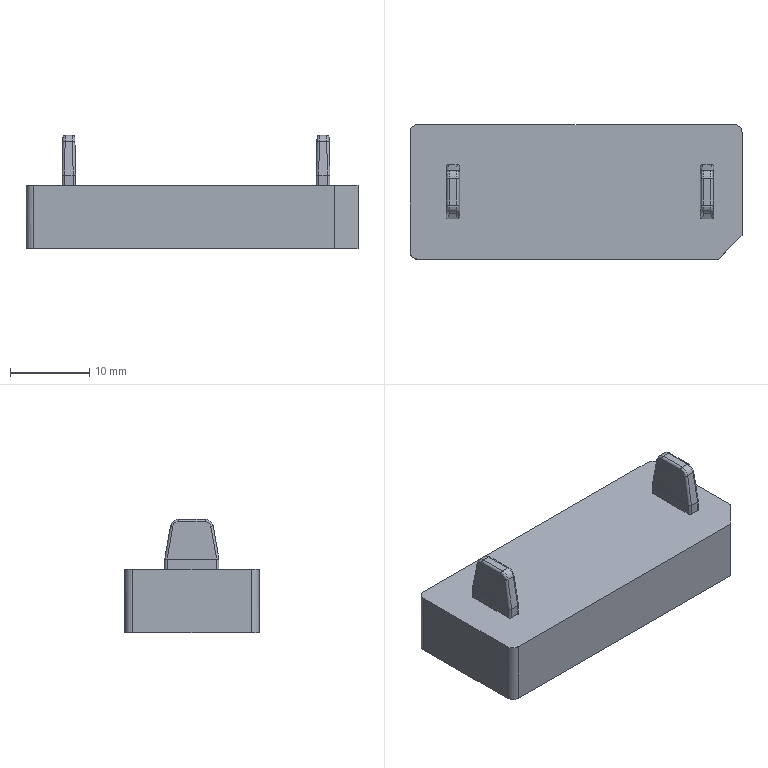NC program | PowerMill | posted by the shop | part box 42 x 17 x 14.346 mm
Lines 1 to 1527 of 86217:
%
G40 G49 G17 G80
( TOOL ID   D10C_1_1 )
( TOOL DIA. 10. TIP RAD 0 LENGTH 69.8 )
( Z = -.074 )
T1 M6
T3
G91 G28 Z0
G0 G90 G54
M08
S8000 M3
G0 X0 Y0 M8
G43 Z10.2 H1
X28.78 Y11.28
Z1.126
G1 Z-.074 F6000
X23.78 F10000
X-23.78
Y5.64
X23.78
Y0
X-23.78
Y-5.64
X23.78
Y-11.28
X-23.78
X-28.78
G0 Z10.2
X.5 Y0
Z9.876
X-29.479 Y-7.144
Z.686
G1 Z-.514 F6000
X-28.951 F10000
G3 X-24.204 Y-2.396 I0 J4.747
G1 Y10.28
G2 X-23.204 Y11.28 I1. J0
G1 X24.204
G2 X25.204 Y10.28 I0 J-1.
G1 Y2.39
X22.604 Y2.224
X22.622 Y1.934
X22.621 Y-1.934
X22.568 Y-2.707
X22.424 Y-3.48
X22.163 Y-4.254
X21.775 Y-5.027
X21.383 Y-5.594
X21.209 Y-5.801
X20.609 Y-6.388
X20.38 Y-6.574
X19.836 Y-6.946
X18.994 Y-7.348
X18.289 Y-7.566
X17.515 Y-7.693
X15.969 Y-7.711
X15.195 Y-7.633
X14.422 Y-7.439
X13.648 Y-7.122
X12.875 Y-6.648
X12.101 Y-5.965
X11.95 Y-5.801
X11.385 Y-5.027
X10.997 Y-4.254
X10.735 Y-3.48
X10.592 Y-2.707
X10.555 Y-2.293
X10.542 Y1.934
X10.587 Y2.707
X10.725 Y3.48
X10.981 Y4.254
X11.328 Y4.969
X11.917 Y5.801
X12.101 Y6.004
X12.875 Y6.686
X13.648 Y7.161
X14.422 Y7.476
X15.195 Y7.673
X15.969 Y7.752
X17.515 Y7.731
X18.289 Y7.605
X19.062 Y7.361
X19.836 Y6.984
X20.609 Y6.427
X21.243 Y5.801
X21.383 Y5.633
X21.799 Y5.027
X22.156 Y4.31
X22.435 Y3.48
X22.573 Y2.707
X22.604 Y2.224
X25.204 Y2.39
Y-10.28
G2 X24.204 Y-11.28 I-1. J0
G1 X-23.204
G2 X-24.204 Y-10.28 I0 J1.
G1 Y-2.396
X-21.599 Y-2.224
X-21.618 Y-1.934
X-21.619 Y1.934
X-21.573 Y2.707
X-21.435 Y3.48
X-21.179 Y4.254
X-20.798 Y5.027
X-20.383 Y5.633
X-20.243 Y5.801
X-19.609 Y6.427
X-19.431 Y6.574
X-18.836 Y6.984
X-18.062 Y7.361
X-17.289 Y7.605
X-16.515 Y7.731
X-14.969 Y7.752
X-14.195 Y7.673
X-13.422 Y7.476
X-13.065 Y7.348
X-12.648 Y7.161
X-11.875 Y6.686
X-11.101 Y6.004
X-10.917 Y5.801
X-10.362 Y5.027
X-9.981 Y4.254
X-9.725 Y3.48
X-9.588 Y2.707
X-9.555 Y2.332
X-9.548 Y-.007
X-3.901 Y-.005
X-3.902 Y3.516
G2 X-1.904 Y5.516 I2. J.001
G1 X2.893 Y5.521
G2 X4.895 Y3.526 I.002 J-2.
G1 X4.91 Y-3.513
G2 X2.913 Y-5.518 I-2. J-.004
G1 X-1.896 Y-5.525
G2 X-3.899 Y-3.526 I-.003 J2.
G1 X-3.901 Y-.005
X-9.548 Y-.007
X-9.542 Y-1.934
X-9.592 Y-2.707
X-9.735 Y-3.48
X-9.997 Y-4.254
X-10.328 Y-4.93
X-10.951 Y-5.801
X-11.101 Y-5.965
X-11.78 Y-6.574
X-12.648 Y-7.122
X-13.166 Y-7.348
X-13.422 Y-7.439
X-14.195 Y-7.633
X-14.969 Y-7.711
X-16.515 Y-7.693
X-17.289 Y-7.566
X-17.991 Y-7.348
X-18.836 Y-6.946
X-19.381 Y-6.574
X-19.609 Y-6.388
X-20.209 Y-5.801
X-20.383 Y-5.594
X-20.775 Y-5.027
X-21.156 Y-4.271
X-21.425 Y-3.48
X-21.567 Y-2.707
X-21.599 Y-2.224
X-24.204 Y-2.396
G0 Z3.296
G1 X-29.479 Y-7.144
G0 Z.296
G1 Z-.904 F6000
X-28.951 F10000
G3 X-24.204 Y-2.396 I0 J4.747
G1 Y0
X-21.619
Y1.934
X-21.618 Y1.951
Y2.707
X-21.512 Y3.48
X-21.3 Y4.254
X-21.156 Y4.618
X-20.953 Y5.027
X-20.45 Y5.801
X-19.722 Y6.574
X-18.836 Y7.208
X-18.581 Y7.348
X-18.062 Y7.581
X-17.289 Y7.817
X-16.515 Y7.942
X-14.969 Y7.961
X-14.195 Y7.883
X-13.422 Y7.694
X-12.648 Y7.383
X-11.875 Y6.917
X-11.438 Y6.574
X-11.101 Y6.255
X-10.71 Y5.801
X-10.207 Y5.027
X-9.859 Y4.254
X-9.649 Y3.48
X-9.555 Y2.861
X-9.531 Y1.934
X-9.537 Y.059
X-3.793 Y.021
X-3.77 Y3.553
G2 X-1.762 Y5.54 I2. J-.013
G1 X2.819 Y5.522
G2 X4.811 Y3.531 I-.008 J-2.
G1 X4.842 Y-3.501
G2 X2.849 Y-5.51 I-2. J-.009
G1 X-1.81 Y-5.526
G2 X-3.817 Y-3.512 I-.007 J2.
G1 X-3.793 Y.021
X-9.537 Y.059
X-9.543 Y-1.621
X-9.542 Y-1.934
X-9.544 Y-1.967
X-9.547 Y-2.707
X-9.657 Y-3.48
X-9.873 Y-4.254
X-10.229 Y-5.027
X-10.741 Y-5.801
X-11.101 Y-6.215
X-11.484 Y-6.574
X-11.875 Y-6.876
X-12.656 Y-7.348
X-13.422 Y-7.655
X-14.195 Y-7.844
X-14.969 Y-7.921
X-16.515 Y-7.903
X-17.289 Y-7.777
X-18.062 Y-7.542
X-18.503 Y-7.348
X-18.836 Y-7.168
X-19.609 Y-6.63
X-20.383 Y-5.847
X-20.931 Y-5.027
X-21.156 Y-4.578
X-21.287 Y-4.254
X-21.504 Y-3.48
X-21.615 Y-2.707
Y-1.986
X-21.618 Y-1.934
X-21.619 Y0
X-24.204
Y10.28
G2 X-23.204 Y11.28 I1. J0
G1 X24.204
G2 X25.204 Y10.28 I0 J-1.
G1 Y2.706
X22.616 Y2.707
Y2.024
X22.622 Y1.934
X22.621 Y-1.934
X22.615 Y-2.015
Y-2.707
X22.503 Y-3.48
X22.285 Y-4.254
X22.156 Y-4.578
X21.931 Y-5.027
X21.419 Y-5.801
X20.676 Y-6.574
X19.836 Y-7.168
X19.504 Y-7.348
X19.062 Y-7.542
X18.289 Y-7.778
X17.515 Y-7.903
X15.969 Y-7.921
X15.195 Y-7.844
X14.422 Y-7.655
X13.656 Y-7.348
X12.875 Y-6.876
X12.484 Y-6.574
X12.101 Y-6.215
X11.741 Y-5.801
X11.229 Y-5.027
X10.873 Y-4.254
X10.657 Y-3.48
X10.545 Y-2.707
X10.543 Y1.887
X10.542 Y1.934
X10.543 Y1.935
X10.542 Y2.707
X10.648 Y3.48
X10.859 Y4.254
X11.207 Y5.027
X11.71 Y5.801
X12.101 Y6.255
X12.438 Y6.574
X12.875 Y6.917
X13.579 Y7.348
X14.422 Y7.694
X15.195 Y7.883
X15.969 Y7.961
X17.515 Y7.942
X18.289 Y7.817
X19.062 Y7.581
X19.582 Y7.348
X19.836 Y7.208
X20.609 Y6.669
X21.383 Y5.887
X21.954 Y5.027
X22.156 Y4.618
X22.301 Y4.254
X22.511 Y3.48
X22.616 Y2.707
X25.204 Y2.706
Y-10.28
G2 X24.204 Y-11.28 I-1. J0
G1 X-23.204
G2 X-24.204 Y-10.28 I0 J1.
G1 Y-2.396
G0 Z2.907
G1 X-29.479 Y-7.144
G0 Z-.093
G1 Z-1.293 F6000
X-28.951 F10000
G3 X-24.204 Y-2.396 I0 J4.747
G1 Y10.28
G2 X-23.204 Y11.28 I1. J0
G1 X24.204
G2 X25.204 Y10.28 I0 J-1.
G1 Y2.706
X22.629 Y2.707
X22.628 Y-2.707
X22.528 Y-3.48
X22.319 Y-4.254
X22.156 Y-4.679
X21.988 Y-5.027
X21.383 Y-5.937
X20.609 Y-6.718
X19.836 Y-7.259
X19.674 Y-7.348
X19.062 Y-7.624
X18.289 Y-7.856
X17.515 Y-7.982
X15.969 Y-8.
X15.195 Y-7.923
X14.422 Y-7.733
X13.648 Y-7.431
X12.875 Y-6.97
X12.388 Y-6.574
X12.101 Y-6.293
X11.669 Y-5.801
X11.328 Y-5.304
X11.172 Y-5.027
X10.841 Y-4.254
X10.632 Y-3.48
X10.532 Y-2.707
X10.53 Y2.707
X10.624 Y3.48
X10.827 Y4.254
X11.152 Y5.027
X11.328 Y5.343
X11.639 Y5.801
X12.101 Y6.333
X12.346 Y6.574
X12.875 Y7.009
X13.413 Y7.348
X13.648 Y7.47
X14.422 Y7.773
X15.195 Y7.962
X15.969 Y8.039
X17.515 Y8.021
X18.289 Y7.895
X19.062 Y7.663
X19.747 Y7.348
X20.609 Y6.757
X20.814 Y6.574
X21.383 Y5.976
X21.521 Y5.801
X22.008 Y5.027
X22.156 Y4.718
X22.333 Y4.254
X22.535 Y3.48
X22.629 Y2.707
X25.204 Y2.706
Y-10.28
G2 X24.204 Y-11.28 I-1. J0
G1 X-23.204
G2 X-24.204 Y-10.28 I0 J1.
G1 Y-2.708
X-21.628 Y-2.707
X-21.63 Y2.707
X-21.535 Y3.48
X-21.333 Y4.254
X-21.156 Y4.718
X-21.009 Y5.027
X-20.521 Y5.801
X-20.383 Y5.976
X-19.814 Y6.574
X-19.609 Y6.757
X-18.836 Y7.298
X-18.062 Y7.663
X-17.289 Y7.895
X-16.515 Y8.021
X-14.969 Y8.039
X-14.195 Y7.962
X-13.422 Y7.773
X-12.648 Y7.47
X-12.413 Y7.348
X-11.875 Y7.009
X-11.346 Y6.574
X-11.101 Y6.333
X-10.639 Y5.801
X-10.328 Y5.343
X-10.152 Y5.027
X-9.827 Y4.254
X-9.624 Y3.48
X-9.53 Y2.707
X-9.531 Y-.021
X-3.807 Y-.011
X-3.813 Y3.501
G2 X-1.817 Y5.505 I2. J.004
G1 X2.793 Y5.515
G2 X4.797 Y3.523 I.004 J-2.
G1 X4.825 Y-3.496
G2 X2.831 Y-5.504 I-2. J-.008
G1 X-1.794 Y-5.519
G2 X-3.801 Y-3.522 I-.007 J2.
G1 X-3.807 Y-.011
X-9.531 Y-.021
X-9.532 Y-2.707
X-9.632 Y-3.48
X-9.841 Y-4.254
X-10.172 Y-5.027
X-10.328 Y-5.304
X-10.669 Y-5.801
X-11.101 Y-6.293
X-11.388 Y-6.574
X-11.875 Y-6.97
X-12.485 Y-7.348
X-13.422 Y-7.733
X-14.195 Y-7.923
X-14.969 Y-8.
X-16.515 Y-7.982
X-17.289 Y-7.856
X-18.062 Y-7.624
X-18.836 Y-7.259
X-19.609 Y-6.718
X-20.383 Y-5.937
X-20.988 Y-5.027
X-21.156 Y-4.679
X-21.32 Y-4.254
X-21.528 Y-3.48
X-21.628 Y-2.707
X-24.204 Y-2.708
Y-2.396
G0 Z2.517
G1 X-29.479 Y-7.144
G0 Z-.483
G1 Z-1.683 F6000
X-28.951 F10000
G3 X-24.204 Y-2.396 I0 J4.747
G1 Y10.28
G2 X-23.204 Y11.28 I1. J0
G1 X24.204
G2 X25.204 Y10.28 I0 J-1.
G1 Y-.001
X22.638 Y0
Y-2.707
X22.548 Y-3.48
X22.348 Y-4.254
X22.156 Y-4.763
X22.03 Y-5.027
X21.55 Y-5.801
X21.383 Y-6.014
X20.852 Y-6.574
X20.609 Y-6.792
X19.807 Y-7.348
X19.062 Y-7.695
X18.289 Y-7.926
X17.515 Y-8.051
X15.969 Y-8.069
X15.195 Y-7.993
X14.422 Y-7.804
X13.648 Y-7.503
X13.353 Y-7.348
X12.875 Y-7.043
X12.308 Y-6.574
X12.101 Y-6.369
X11.61 Y-5.801
X11.328 Y-5.384
X11.13 Y-5.027
X10.812 Y-4.254
X10.613 Y-3.48
X10.555 Y-3.113
X10.523 Y-2.707
X10.521 Y2.707
X10.606 Y3.48
X10.799 Y4.254
X11.11 Y5.027
X11.328 Y5.423
X11.581 Y5.801
X12.267 Y6.574
X12.875 Y7.083
X13.284 Y7.348
X13.648 Y7.542
X14.422 Y7.843
X15.195 Y8.032
X15.969 Y8.108
X17.515 Y8.09
X18.289 Y7.965
X19.062 Y7.734
X19.836 Y7.371
X20.609 Y6.831
X20.893 Y6.574
X21.383 Y6.053
X21.579 Y5.801
X22.05 Y5.027
X22.361 Y4.254
X22.554 Y3.48
X22.639 Y2.707
X22.638 Y0
X25.204 Y-.001
Y-10.28
G2 X24.204 Y-11.28 I-1. J0
G1 X-23.204
G2 X-24.204 Y-10.28 I0 J1.
G1 Y-2.708
X-21.638 Y-2.707
X-21.639 Y2.707
X-21.555 Y3.48
X-21.361 Y4.254
X-21.051 Y5.027
X-20.579 Y5.801
X-20.383 Y6.053
X-19.893 Y6.574
X-19.609 Y6.831
X-18.876 Y7.348
X-18.062 Y7.734
X-17.289 Y7.965
X-16.515 Y8.09
X-14.969 Y8.108
X-14.195 Y8.032
X-13.422 Y7.843
X-12.648 Y7.542
X-12.285 Y7.348
X-11.875 Y7.083
X-11.267 Y6.574
X-10.581 Y5.801
X-10.328 Y5.423
X-10.11 Y5.027
X-9.799 Y4.254
X-9.605 Y3.48
X-9.521 Y2.707
Y-.019
X-3.779 Y-.01
X-3.785 Y3.505
G2 X-1.785 Y5.508 I2. J.003
G1 X2.785
G2 X4.785 Y3.512 I0 J-2.
G1 X4.798 Y-3.503
G2 X2.804 Y-5.506 I-2. J-.004
G1 X-1.767 Y-5.521
G2 X-3.774 Y-3.525 I-.007 J2.
G1 X-3.779 Y-.01
X-9.521 Y-.019
X-9.522 Y-2.707
X-9.555 Y-3.113
X-9.613 Y-3.48
X-9.812 Y-4.254
X-10.13 Y-5.027
X-10.328 Y-5.384
X-10.61 Y-5.801
X-11.101 Y-6.369
X-11.307 Y-6.574
X-11.875 Y-7.043
X-12.354 Y-7.348
X-12.648 Y-7.503
X-13.422 Y-7.804
X-14.195 Y-7.993
X-14.969 Y-8.069
X-16.515 Y-8.051
X-17.289 Y-7.926
X-18.062 Y-7.695
X-18.836 Y-7.332
X-19.609 Y-6.792
X-19.852 Y-6.574
X-20.383 Y-6.014
X-20.55 Y-5.801
X-21.03 Y-5.027
X-21.156 Y-4.763
X-21.348 Y-4.254
X-21.548 Y-3.48
X-21.638 Y-2.707
X-24.204 Y-2.708
Y-2.396
G0 Z2.127
G1 X-29.479 Y-7.144
G0 Z-.873
G1 Z-2.073 F6000
X-28.951 F10000
G3 X-24.204 Y-2.396 I0 J4.747
G1 Y10.28
G2 X-23.204 Y11.28 I1. J0
G1 X24.204
G2 X25.204 Y10.28 I0 J-1.
G1 Y-.001
X22.648 Y0
X22.646 Y-2.707
X22.567 Y-3.48
X22.376 Y-4.254
X22.072 Y-5.027
X21.607 Y-5.801
X21.383 Y-6.09
X20.929 Y-6.574
X20.609 Y-6.866
X19.932 Y-7.348
X19.062 Y-7.766
X18.289 Y-7.996
X17.505 Y-8.121
X15.969 Y-8.138
X15.195 Y-8.062
X14.422 Y-7.875
X13.648 Y-7.575
X13.228 Y-7.348
X12.875 Y-7.117
X12.23 Y-6.574
X11.553 Y-5.801
X11.328 Y-5.463
X11.088 Y-5.027
X10.784 Y-4.254
X10.594 Y-3.48
X10.557 Y-3.128
X10.555 Y-3.113
X10.552 Y-3.08
X10.513 Y-2.707
Y-.033
X4.734 Y-.012
X4.722 Y-3.538
G2 X2.71 Y-5.531 I-2. J.007
G1 X-1.787 Y-5.505
G2 X-3.776 Y-3.505 I.011 J2.
G1 X-3.773 Y3.502
G2 X-1.782 Y5.501 I2. J-.001
G1 X2.739 Y5.521
G2 X4.747 Y3.513 I.009 J-2.
G1 X4.734 Y-.012
X10.513 Y-.033
X10.512 Y2.707
X10.555 Y3.275
X10.771 Y4.254
X11.069 Y5.027
X11.328 Y5.503
X11.525 Y5.801
X12.101 Y6.484
X12.875 Y7.156
X13.164 Y7.348
X13.648 Y7.614
X14.422 Y7.914
X15.195 Y8.102
X15.969 Y8.177
X17.515 Y8.159
X18.289 Y8.035
X19.062 Y7.805
X19.836 Y7.444
X20.609 Y6.906
X20.968 Y6.574
X21.383 Y6.129
X21.635 Y5.801
X22.091 Y5.027
X22.389 Y4.254
X22.574 Y3.48
X22.649 Y2.707
X22.648 Y0
X25.204 Y-.001
Y-10.28
G2 X24.204 Y-11.28 I-1. J0
G1 X-23.204
G2 X-24.204 Y-10.28 I0 J1.
G1 Y-2.707
X-21.647
X-21.648 Y2.707
X-21.574 Y3.48
X-21.389 Y4.254
X-21.156 Y4.886
X-20.635 Y5.801
X-20.383 Y6.129
X-19.969 Y6.574
X-19.609 Y6.906
X-18.836 Y7.444
X-18.062 Y7.805
X-17.289 Y8.035
X-16.515 Y8.159
X-14.969 Y8.177
X-14.315 Y8.121
X-13.422 Y7.914
X-12.648 Y7.614
X-12.163 Y7.348
X-11.875 Y7.156
X-11.192 Y6.574
X-10.525 Y5.801
X-10.328 Y5.503
X-10.069 Y5.027
X-9.771 Y4.254
X-9.586 Y3.48
X-9.511 Y2.707
X-9.512 Y-2.707
X-9.554 Y-3.099
X-9.555 Y-3.113
X-9.556 Y-3.119
X-9.593 Y-3.48
X-9.783 Y-4.254
X-10.088 Y-5.027
X-10.328 Y-5.463
X-10.553 Y-5.801
X-11.101 Y-6.445
X-11.875 Y-7.117
X-12.228 Y-7.348
X-12.648 Y-7.575
X-13.422 Y-7.875
X-14.195 Y-8.062
X-14.654 Y-8.121
X-14.969 Y-8.138
X-16.505 Y-8.121
X-17.289 Y-7.996
X-18.062 Y-7.766
X-18.836 Y-7.404
X-19.609 Y-6.866
X-19.929 Y-6.574
X-20.383 Y-6.09
X-20.607 Y-5.801
X-21.071 Y-5.027
X-21.377 Y-4.254
X-21.567 Y-3.48
X-21.647 Y-2.707
X-24.204
Y-2.396
G0 Z1.737
G1 X-29.479 Y-7.144
G0 Z-1.263
G1 Z-2.463 F6000
X-28.951 F10000
G3 X-24.204 Y-2.396 I0 J4.747
G1 Y0
X-21.656
Y2.707
X-21.592 Y3.48
X-21.415 Y4.254
X-21.156 Y4.97
X-20.691 Y5.801
X-20.383 Y6.206
X-20.044 Y6.574
X-19.609 Y6.98
X-19.111 Y7.348
X-18.836 Y7.516
X-18.062 Y7.877
X-17.289 Y8.106
X-16.515 Y8.229
X-14.969 Y8.246
X-14.195 Y8.172
X-13.422 Y7.985
X-12.648 Y7.686
X-11.875 Y7.23
X-11.101 Y6.56
X-10.47 Y5.801
X-10.328 Y5.582
X-10.031 Y5.027
X-9.745 Y4.254
X-9.567 Y3.48
X-9.504 Y2.707
Y-2.707
X-9.555 Y-3.355
X-9.756 Y-4.254
X-10.049 Y-5.027
X-10.328 Y-5.543
X-10.497 Y-5.801
X-11.101 Y-6.52
X-11.875 Y-7.19
X-12.109 Y-7.348
X-12.648 Y-7.647
X-13.422 Y-7.946
X-14.132 Y-8.121
X-14.969 Y-8.206
X-16.515 Y-8.189
X-17.289 Y-8.067
X-18.062 Y-7.837
X-18.836 Y-7.477
X-19.051 Y-7.348
X-19.609 Y-6.941
X-20.005 Y-6.574
X-20.383 Y-6.167
X-20.663 Y-5.801
X-21.111 Y-5.027
X-21.405 Y-4.254
X-21.586 Y-3.48
X-21.656 Y-2.707
Y0
X-24.204
Y10.28
G2 X-23.204 Y11.28 I1. J0
G1 X24.204
G2 X25.204 Y10.28 I0 J-1.
G1 Y0
X22.656
X22.655 Y-2.707
X22.586 Y-3.48
X22.405 Y-4.254
X22.156 Y-4.931
X21.663 Y-5.801
X21.383 Y-6.167
X21.005 Y-6.574
X20.609 Y-6.941
X20.051 Y-7.348
X19.836 Y-7.477
X19.062 Y-7.837
X18.289 Y-8.067
X18.028 Y-8.121
X17.515 Y-8.189
X15.969 Y-8.206
X15.195 Y-8.132
X14.422 Y-7.946
X13.648 Y-7.647
X13.109 Y-7.348
X12.875 Y-7.19
X12.155 Y-6.574
X11.497 Y-5.801
X11.328 Y-5.543
X11.049 Y-5.027
X10.755 Y-4.254
X10.575 Y-3.48
X10.504 Y-2.707
Y.089
X4.73 Y.033
X4.764 Y-3.479
G2 X2.764 Y-5.498 I-2. J-.019
G1 X-1.769
G2 X-3.769 Y-3.496 I0 J2.
G1 X-3.762 Y3.496
G2 X-1.776 Y5.494 I2. J-.002
G1 X2.682 Y5.525
G2 X4.696 Y3.545 I.014 J-2.
G1 X4.73 Y.033
X10.504 Y.089
Y2.707
X10.555 Y3.395
X10.745 Y4.254
X11.031 Y5.027
X11.328 Y5.582
X11.47 Y5.801
X12.101 Y6.56
X12.875 Y7.23
X13.648 Y7.686
X14.422 Y7.985
X15.195 Y8.172
X15.969 Y8.246
X17.515 Y8.229
X18.222 Y8.121
X19.062 Y7.877
X19.836 Y7.516
X20.112 Y7.348
X20.609 Y6.98
X21.043 Y6.574
X21.383 Y6.206
X21.69 Y5.801
X22.13 Y5.027
X22.415 Y4.254
X22.592 Y3.48
X22.656 Y2.707
Y0
X25.204
Y-10.28
G2 X24.204 Y-11.28 I-1. J0
G1 X-23.204
G2 X-24.204 Y-10.28 I0 J1.
G1 Y-2.396
G0 Z1.348
G1 X-29.479 Y-7.144
G0 Z-1.652
G1 Z-2.852 F6000
X-28.951 F10000
G3 X-24.204 Y-2.396 I0 J4.747
G1 Y10.28
G2 X-23.204 Y11.28 I1. J0
G1 X24.204
G2 X25.204 Y10.28 I0 J-1.
G1 Y0
X22.663
Y-2.707
X22.603 Y-3.48
X22.43 Y-4.254
X22.156 Y-5.015
X21.717 Y-5.801
X21.383 Y-6.244
X21.079 Y-6.574
X20.609 Y-7.015
X20.163 Y-7.348
X19.836 Y-7.549
X19.062 Y-7.909
X18.354 Y-8.121
X17.515 Y-8.259
X15.969 Y-8.275
X15.195 Y-8.202
X14.422 Y-8.016
X13.648 Y-7.719
X12.996 Y-7.348
X12.101 Y-6.596
X11.443 Y-5.801
X11.01 Y-5.027
X10.73 Y-4.254
X10.556 Y-3.48
X10.497 Y-2.707
Y2.707
X10.555 Y3.51
X10.719 Y4.254
X10.992 Y5.027
X11.417 Y5.801
X12.042 Y6.574
X12.875 Y7.303
X13.648 Y7.758
X14.422 Y8.056
X15.195 Y8.241
X15.969 Y8.314
X17.515 Y8.298
X18.289 Y8.176
X19.062 Y7.948
X19.836 Y7.589
X20.221 Y7.348
X20.609 Y7.054
X21.117 Y6.574
X21.383 Y6.283
X21.743 Y5.801
X22.156 Y5.054
X22.441 Y4.254
X22.609 Y3.48
X22.663 Y2.707
Y0
X25.204
Y-10.28
G2 X24.204 Y-11.28 I-1. J0
G1 X-23.204
G2 X-24.204 Y-10.28 I0 J1.
G1 Y-2.707
X-21.663
Y2.707
X-21.609 Y3.48
X-21.441 Y4.254
X-21.168 Y5.027
X-20.743 Y5.801
X-20.383 Y6.283
X-20.118 Y6.574
X-19.609 Y7.054
X-19.221 Y7.348
X-18.836 Y7.589
X-18.062 Y7.948
X-17.289 Y8.176
X-16.515 Y8.298
X-14.969 Y8.314
X-14.195 Y8.241
X-13.422 Y8.056
X-12.648 Y7.758
X-11.939 Y7.348
X-11.101 Y6.635
X-10.417 Y5.801
X-9.993 Y5.027
X-9.72 Y4.254
X-9.555 Y3.51
X-9.497 Y2.707
Y-.045
X-3.691 Y-.021
X-3.705 Y3.491
G2 X-1.707 Y5.515 I2. J.024
G1 X2.676 Y5.52
G2 X4.678 Y3.541 I.002 J-2.
G1 X4.753 Y-3.47
G2 X2.77 Y-5.491 I-2. J-.021
G1 X-1.659 Y-5.528
G2 X-3.676 Y-3.533 I-.017 J2.
G1 X-3.691 Y-.021
X-9.497 Y-.045
Y-2.707
X-9.555 Y-3.471
X-9.729 Y-4.254
X-10.011 Y-5.027
X-10.443 Y-5.801
X-11.101 Y-6.596
X-11.875 Y-7.264
X-12.648 Y-7.719
X-13.422 Y-8.016
X-13.807 Y-8.121
X-14.195 Y-8.202
X-14.969 Y-8.275
X-16.515 Y-8.259
X-17.289 Y-8.137
X-18.062 Y-7.909
X-18.836 Y-7.549
X-19.164 Y-7.348
X-19.609 Y-7.015
X-20.08 Y-6.574
X-20.383 Y-6.244
X-20.716 Y-5.801
X-21.15 Y-5.027
X-21.43 Y-4.254
X-21.604 Y-3.48
X-21.663 Y-2.707
X-24.204
Y-2.396
G0 Z.958
G1 X-29.479 Y-7.144
G0 Z-2.042
G1 Z-3.242 F6000
X-28.951 F10000
G3 X-24.204 Y-2.396 I0 J4.747
G1 Y10.28
G2 X-23.204 Y11.28 I1. J0
G1 X24.204
G2 X25.204 Y10.28 I0 J-1.
G1 Y0
X22.67
Y-2.707
X22.62 Y-3.48
X22.455 Y-4.254
X22.187 Y-5.027
X21.769 Y-5.801
X21.383 Y-6.321
X21.153 Y-6.574
X20.609 Y-7.089
X20.27 Y-7.348
X19.836 Y-7.622
X19.062 Y-7.98
X18.618 Y-8.121
X18.289 Y-8.207
X17.515 Y-8.328
X15.969 Y-8.344
X15.195 Y-8.272
X14.542 Y-8.121
X13.648 Y-7.79
X12.89 Y-7.348
X12.101 Y-6.672
X11.39 Y-5.801
X10.973 Y-5.027
X10.704 Y-4.254
X10.555 Y-3.584
X10.49 Y-2.707
Y2.707
X10.535 Y3.48
X10.694 Y4.254
X10.956 Y5.027
X11.328 Y5.741
X11.969 Y6.574
X12.834 Y7.348
X13.648 Y7.83
X14.404 Y8.121
X15.195 Y8.311
X15.969 Y8.383
X17.515 Y8.367
X18.289 Y8.246
X19.062 Y8.019
X19.836 Y7.661
X20.326 Y7.348
X20.609 Y7.129
X21.191 Y6.574
X21.383 Y6.36
X21.795 Y5.801
X22.156 Y5.138
X22.466 Y4.254
X22.626 Y3.48
X22.67 Y2.707
Y0
X25.204
Y-10.28
G2 X24.204 Y-11.28 I-1. J0
G1 X-23.204
G2 X-24.204 Y-10.28 I0 J1.
G1 Y-3.163
X-21.651 Y-2.997
X-21.67 Y-2.707
Y2.707
X-21.626 Y3.48
X-21.466 Y4.254
X-21.204 Y5.027
X-20.795 Y5.801
X-20.383 Y6.36
X-20.191 Y6.574
X-19.609 Y7.129
X-19.326 Y7.348
X-18.836 Y7.661
X-18.062 Y8.019
X-17.289 Y8.246
X-16.515 Y8.367
X-14.969 Y8.383
X-14.195 Y8.311
X-13.422 Y8.126
X-12.648 Y7.83
X-11.875 Y7.377
X-10.969 Y6.574
X-10.365 Y5.801
X-9.956 Y5.027
X-9.694 Y4.254
X-9.555 Y3.622
X-9.49 Y2.707
Y-.055
X-3.717 Y-.025
X-3.735 Y3.47
G2 X-1.747 Y5.481 I2. J.01
G1 X2.685 Y5.507
G2 X4.696 Y3.519 I.012 J-2.
G1 X4.739 Y-3.472
G2 X2.751 Y-5.484 I-2. J-.012
G1 X-1.687 Y-5.51
G2 X-3.699 Y-3.521 I-.012 J2.
G1 X-3.717 Y-.025
X-9.49 Y-.055
Y-2.707
X-9.54 Y-3.48
X-9.704 Y-4.254
X-9.972 Y-5.027
X-10.328 Y-5.702
X-11.007 Y-6.574
X-11.875 Y-7.337
X-12.648 Y-7.79
X-13.542 Y-8.121
X-14.195 Y-8.272
X-14.969 Y-8.344
X-16.515 Y-8.328
X-17.289 Y-8.207
X-18.062 Y-7.98
X-18.836 Y-7.622
X-19.27 Y-7.348
X-19.609 Y-7.089
X-20.153 Y-6.574
X-20.383 Y-6.321
X-20.77 Y-5.801
X-21.156 Y-5.099
X-21.456 Y-4.254
X-21.62 Y-3.48
X-21.651 Y-2.997
X-24.204 Y-3.163
Y-2.396
G0 Z.568
G1 X-29.479 Y-7.144
G0 Z-2.432
G1 Z-3.632 F6000
X-28.951 F10000
G3 X-24.204 Y-2.396 I0 J4.747
G1 Y0
X-21.677
Y2.707
X-21.641 Y3.48
X-21.491 Y4.254
X-21.239 Y5.027
X-20.845 Y5.801
X-20.383 Y6.437
X-19.609 Y7.203
X-19.425 Y7.348
X-18.836 Y7.734
X-18.062 Y8.09
X-17.289 Y8.317
X-16.515 Y8.436
X-14.969 Y8.452
X-14.195 Y8.381
X-13.422 Y8.197
X-12.648 Y7.902
X-11.875 Y7.45
X-11.101 Y6.786
X-10.899 Y6.574
X-10.315 Y5.801
X-9.921 Y5.027
X-9.669 Y4.254
X-9.519 Y3.48
X-9.483 Y2.707
Y-2.707
X-9.524 Y-3.48
X-9.679 Y-4.254
X-9.937 Y-5.027
X-10.34 Y-5.801
X-10.935 Y-6.574
X-11.101 Y-6.747
X-11.787 Y-7.348
X-12.648 Y-7.862
X-13.302 Y-8.121
X-14.195 Y-8.342
X-14.969 Y-8.413
X-16.515 Y-8.397
X-17.289 Y-8.277
X-18.062 Y-8.051
X-18.836 Y-7.695
X-19.373 Y-7.348
X-19.609 Y-7.164
X-20.226 Y-6.574
X-20.383 Y-6.397
X-20.82 Y-5.801
X-21.156 Y-5.182
X-21.481 Y-4.254
X-21.636 Y-3.48
X-21.677 Y-2.707
Y0
X-24.204
Y10.28
G2 X-23.204 Y11.28 I1. J0
G1 X24.204
G2 X25.204 Y10.28 I0 J-1.
G1 Y0
X22.677
Y-2.707
X22.637 Y-3.48
X22.48 Y-4.254
X22.223 Y-5.027
X21.82 Y-5.801
X21.383 Y-6.397
X21.225 Y-6.574
X20.609 Y-7.164
X20.374 Y-7.348
X19.836 Y-7.695
X19.062 Y-8.051
X18.858 Y-8.121
X18.289 Y-8.277
X17.515 Y-8.397
X15.969 Y-8.413
X15.195 Y-8.342
X14.422 Y-8.158
X13.648 Y-7.862
X12.875 Y-7.411
X12.101 Y-6.747
X11.935 Y-6.574
X11.34 Y-5.801
X10.937 Y-5.027
X10.679 Y-4.254
X10.524 Y-3.48
X10.483 Y-2.707
Y2.707
X10.52 Y3.48
X10.668 Y4.254
X10.921 Y5.027
X11.315 Y5.801
X11.898 Y6.574
X12.101 Y6.786
X12.875 Y7.45
X13.648 Y7.902
X14.184 Y8.121
X15.195 Y8.381
X15.969 Y8.452
X17.515 Y8.436
X18.289 Y8.317
X18.976 Y8.121
X19.836 Y7.734
X20.426 Y7.348
X20.609 Y7.203
X21.261 Y6.574
X21.845 Y5.801
X22.24 Y5.027
X22.492 Y4.254
X22.64 Y3.48
X22.677 Y2.707
Y0
X25.204
Y-10.28
G2 X24.204 Y-11.28 I-1. J0
G1 X-1.639
X-1.658 Y-5.518
G2 X-3.665 Y-3.514 I-.007 J2.
G1 X-3.651 Y3.516
G2 X-1.644 Y5.512 I2. J-.004
G1 X2.691 Y5.499
G2 X4.685 Y3.5 I-.006 J-2.
G1 X4.687 Y-3.502
G2 X2.694 Y-5.503 I-2. J-.001
G1 X-1.658 Y-5.518
X-1.639 Y-11.28
X-23.204
G2 X-24.204 Y-10.28 I0 J1.
G1 Y-2.396
G0 Z.178
G1 X-29.479 Y-7.144
G0 Z-2.822
G1 Z-4.022 F6000
X-28.951 F10000
G3 X-24.204 Y-2.396 I0 J4.747
G1 Y0
X-21.684
Y2.707
X-21.656 Y3.48
X-21.517 Y4.254
X-21.275 Y5.027
X-21.156 Y5.304
X-20.893 Y5.801
X-20.383 Y6.513
X-19.609 Y7.277
X-18.836 Y7.806
X-18.169 Y8.121
X-17.289 Y8.387
X-16.515 Y8.506
X-14.969 Y8.521
X-14.195 Y8.451
X-13.422 Y8.268
X-12.99 Y8.121
X-12.648 Y7.974
X-11.875 Y7.524
X-11.639 Y7.348
X-11.101 Y6.862
X-10.83 Y6.574
X-10.328 Y5.901
X-9.886 Y5.027
X-9.644 Y4.254
X-9.555 Y3.842
X-9.505 Y3.48
X-9.476 Y2.707
Y-2.707
X-9.509 Y-3.48
X-9.654 Y-4.254
X-9.902 Y-5.027
X-10.29 Y-5.801
X-10.865 Y-6.574
X-11.101 Y-6.823
X-11.689 Y-7.348
X-11.875 Y-7.485
X-12.648 Y-7.934
X-13.094 Y-8.121
X-13.422 Y-8.229
X-14.195 Y-8.412
X-14.969 Y-8.482
X-16.515 Y-8.466
X-17.289 Y-8.348
X-18.065 Y-8.121
X-18.836 Y-7.767
X-19.472 Y-7.348
X-20.294 Y-6.574
X-20.87 Y-5.801
X-21.156 Y-5.265
X-21.259 Y-5.027
X-21.506 Y-4.254
X-21.651 Y-3.48
X-21.684 Y-2.707
Y0
X-24.204
Y10.28
G2 X-23.204 Y11.28 I1. J0
G1 X24.204
G2 X25.204 Y10.28 I0 J-1.
G1 Y2.899
X22.68 Y2.804
X22.684 Y2.707
Y-2.707
X22.651 Y-3.48
X22.505 Y-4.254
X22.259 Y-5.027
X21.87 Y-5.801
X21.383 Y-6.474
X20.609 Y-7.238
X19.836 Y-7.767
X19.065 Y-8.121
X18.289 Y-8.348
X17.515 Y-8.466
X15.969 Y-8.482
X15.195 Y-8.412
X14.422 Y-8.229
X14.095 Y-8.121
X13.648 Y-7.934
X12.875 Y-7.485
X12.689 Y-7.348
X12.101 Y-6.823
X11.865 Y-6.574
X11.328 Y-5.861
X10.901 Y-5.027
X10.654 Y-4.254
X10.509 Y-3.48
X10.476 Y-2.707
Y.031
X4.664 Y.011
X4.676 Y-3.489
G2 X2.682 Y-5.496 I-2. J-.007
G1 X-1.647 Y-5.51
G2 X-3.654 Y-3.515 I-.006 J2.
G1 X-3.672 Y3.484
G2 X-1.679 Y5.489 I2. J.005
G1 X2.645 Y5.505
G2 X4.652 Y3.512 I.007 J-2.
G1 X4.664 Y.011
X10.476 Y.031
Y2.707
X10.505 Y3.48
X10.644 Y4.254
X10.885 Y5.027
X11.267 Y5.801
X11.831 Y6.574
X12.101 Y6.862
X12.638 Y7.348
X12.875 Y7.524
X13.648 Y7.974
X13.99 Y8.121
X14.422 Y8.268
X15.195 Y8.451
X15.969 Y8.521
X17.515 Y8.506
X18.289 Y8.387
X19.062 Y8.162
X19.836 Y7.806
X20.521 Y7.348
X21.33 Y6.574
X21.893 Y5.801
X22.156 Y5.304
X22.274 Y5.027
X22.516 Y4.254
X22.655 Y3.48
X22.68 Y2.804
X25.204 Y2.899
Y-10.28
G2 X24.204 Y-11.28 I-1. J0
G1 X-23.204
G2 X-24.204 Y-10.28 I0 J1.
G1 Y-2.396
G0 Z-.211
G1 X-29.479 Y-7.144
G0 Z-3.211
G1 Z-4.411 F6000
X-28.951 F10000
G3 X-24.204 Y-2.396 I0 J4.747
G1 Y0
X-21.691
Y2.707
X-21.668 Y3.48
X-21.54 Y4.254
X-21.307 Y5.027
X-21.156 Y5.388
X-20.941 Y5.801
X-20.383 Y6.59
X-19.614 Y7.348
X-18.836 Y7.879
X-18.344 Y8.121
X-18.062 Y8.233
X-17.289 Y8.457
X-16.515 Y8.575
X-14.969 Y8.59
X-14.195 Y8.521
X-13.422 Y8.339
X-12.648 Y8.046
X-11.875 Y7.597
X-11.546 Y7.348
X-11.101 Y6.938
X-10.765 Y6.574
X-10.219 Y5.801
X-9.852 Y5.027
X-9.619 Y4.254
X-9.492 Y3.48
X-9.469 Y2.707
Y-2.707
X-9.495 Y-3.48
X-9.555 Y-3.91
X-9.63 Y-4.254
X-9.867 Y-5.027
X-10.242 Y-5.801
X-10.798 Y-6.574
X-11.101 Y-6.898
X-11.595 Y-7.348
X-11.875 Y-7.558
X-12.648 Y-8.006
X-12.91 Y-8.121
X-13.422 Y-8.299
X-14.195 Y-8.482
X-14.969 Y-8.551
X-16.515 Y-8.536
X-17.289 Y-8.418
X-18.062 Y-8.194
X-18.836 Y-7.84
X-19.565 Y-7.348
X-20.363 Y-6.574
X-20.918 Y-5.801
X-21.156 Y-5.349
X-21.293 Y-5.027
X-21.53 Y-4.254
X-21.665 Y-3.48
X-21.691 Y-2.707
Y0
X-24.204
Y10.28
G2 X-23.204 Y11.28 I1. J0
G1 X24.204
G2 X25.204 Y10.28 I0 J-1.
G1 Y3.552
X22.669 Y3.48
X22.691 Y2.707
Y-2.707
X22.664 Y-3.48
X22.53 Y-4.254
X22.292 Y-5.027
X22.156 Y-5.349
X21.918 Y-5.801
X21.383 Y-6.551
X20.609 Y-7.313
X19.836 Y-7.84
X19.251 Y-8.121
X18.289 Y-8.418
X17.515 Y-8.536
X15.969 Y-8.551
X15.195 Y-8.482
X14.422 Y-8.299
X13.648 Y-8.006
X12.875 Y-7.558
X12.595 Y-7.348
X12.101 Y-6.898
X11.799 Y-6.574
X11.328 Y-5.941
X10.867 Y-5.027
X10.63 Y-4.254
X10.555 Y-3.91
X10.496 Y-3.48
X10.469 Y-2.707
Y.05
X4.645 Y.02
X4.663 Y-3.476
G2 X2.669 Y-5.486 I-2. J-.01
G1 X-1.635 Y-5.499
G2 X-3.641 Y-3.505 I-.006 J2.
G1 X-3.661 Y3.479
G2 X-1.671 Y5.484 I2. J.006
G1 X2.616 Y5.506
G2 X4.627 Y3.516 I.01 J-2.
G1 X4.645 Y.02
X10.469 Y.05
Y2.707
X10.492 Y3.48
X10.62 Y4.254
X10.853 Y5.027
X11.219 Y5.801
X11.764 Y6.574
X12.101 Y6.938
X12.546 Y7.348
X12.875 Y7.597
X13.648 Y8.046
X14.422 Y8.339
X15.195 Y8.521
X15.969 Y8.59
X17.515 Y8.575
X18.289 Y8.457
X19.062 Y8.233
X19.344 Y8.121
X19.836 Y7.879
X20.609 Y7.352